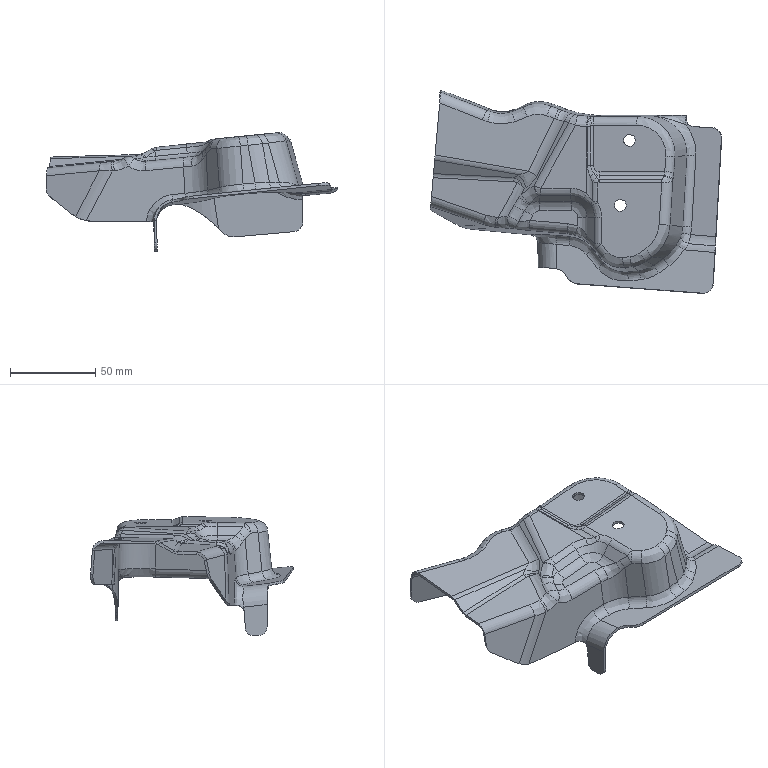Part | 1 solid | 329 faces | box 171.16 x 119.236 x 69.7 mm | volume 38707 mm3 | spline 194 | cylinder 94 | plane 34 | sphere 4 | other 3 | commonest cylinder face diameters 10 x15 9 x12 12 x12 13 x11 7 x10 16 x4